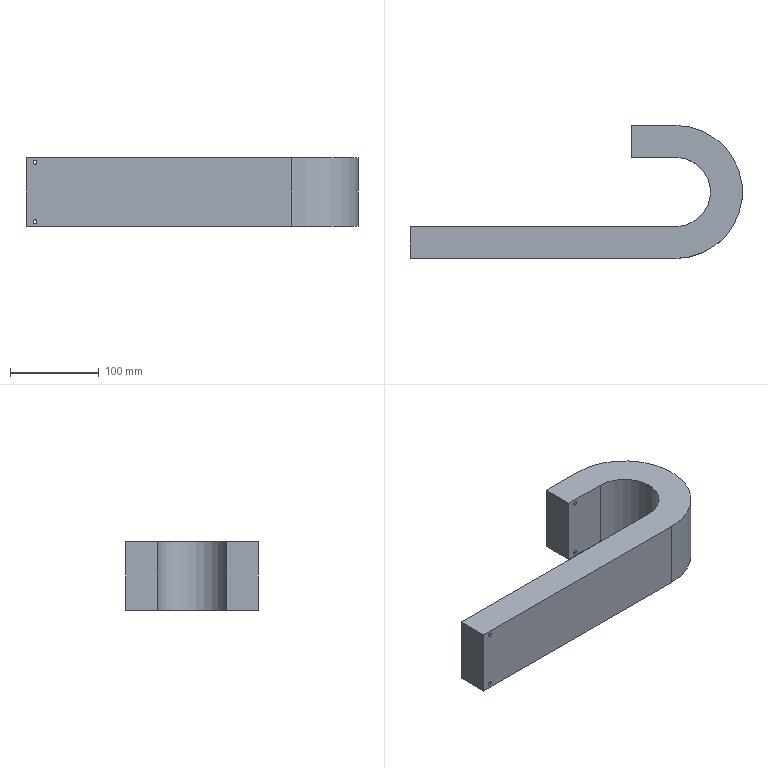Part | STEP file | 1 solid | 18 faces | box 375 x 150 x 77.5 mm | volume 1474112 mm3 | cylinder 10 | plane 8 | commonest cylinder face diameters 4.2 x8 78 x1 150 x1
STEP:
#1=CARTESIAN_POINT('',(0.,0.,0.));
#2=DIRECTION('',(0.,0.,1.));
#3=DIRECTION('',(1.,0.,0.));
#4=AXIS2_PLACEMENT_3D('',#1,#2,#3);
#5=CARTESIAN_POINT('',(-240.,36.,31.4));
#6=VERTEX_POINT('',#5);
#7=CARTESIAN_POINT('',(-240.,0.,31.4));
#8=VERTEX_POINT('',#7);
#9=CARTESIAN_POINT('',(-240.,0.,31.4));
#10=DIRECTION('',(0.,-1.,0.));
#11=VECTOR('',#10,1.);
#12=LINE('',#9,#11);
#13=CARTESIAN_POINT('',(-240.,0.,33.5));
#14=DIRECTION('',(0.,-1.,0.));
#15=DIRECTION('',(0.,0.,-1.));
#16=AXIS2_PLACEMENT_3D('',#13,#14,#15);
#17=CYLINDRICAL_SURFACE('',#16,2.1);
#18=CARTESIAN_POINT('',(6.283,0.));
#19=DIRECTION('',(0.,1.));
#20=VECTOR('',#19,1.);
#21=LINE('',#18,#20);
#22=(GEOMETRIC_REPRESENTATION_CONTEXT(2)PARAMETRIC_REPRESENTATION_CONTEXT()REPRESENTATION_CONTEXT('',''));
#23=DEFINITIONAL_REPRESENTATION('',(#21),#22);
#24=PCURVE('',#17,#23);
#25=CARTESIAN_POINT('',(-240.,0.,33.5));
#26=DIRECTION('',(0.,-1.,0.));
#27=DIRECTION('',(0.,0.,-1.));
#28=AXIS2_PLACEMENT_3D('',#25,#26,#27);
#29=CYLINDRICAL_SURFACE('',#28,2.1);
#30=CARTESIAN_POINT('',(0.,0.));
#31=DIRECTION('',(0.,1.));
#32=VECTOR('',#31,1.);
#33=LINE('',#30,#32);
#34=(GEOMETRIC_REPRESENTATION_CONTEXT(2)PARAMETRIC_REPRESENTATION_CONTEXT()REPRESENTATION_CONTEXT('',''));
#35=DEFINITIONAL_REPRESENTATION('',(#33),#34);
#36=PCURVE('',#29,#35);
#37=SURFACE_CURVE('',#12,(#24,#36),.PCURVE_S1.);
#38=EDGE_CURVE('',#6,#8,#37,.T.);
#39=ORIENTED_EDGE('',*,*,#38,.T.);
#40=CARTESIAN_POINT('',(-240.,0.,35.6));
#41=VERTEX_POINT('',#40);
#42=CARTESIAN_POINT('',(-240.,0.,33.5));
#43=DIRECTION('',(0.,-1.,0.));
#44=DIRECTION('',(0.,0.,-1.));
#45=AXIS2_PLACEMENT_3D('',#42,#43,#44);
#46=CIRCLE('',#45,2.1);
#47=CARTESIAN_POINT('',(0.,0.));
#48=DIRECTION('',(1.,0.));
#49=VECTOR('',#48,1.);
#50=LINE('',#47,#49);
#51=(GEOMETRIC_REPRESENTATION_CONTEXT(2)PARAMETRIC_REPRESENTATION_CONTEXT()REPRESENTATION_CONTEXT('',''));
#52=DEFINITIONAL_REPRESENTATION('',(#50),#51);
#53=PCURVE('',#17,#52);
#54=CARTESIAN_POINT('',(-250.,0.,38.75));
#55=DIRECTION('',(0.,1.,0.));
#56=DIRECTION('',(0.,0.,1.));
#57=AXIS2_PLACEMENT_3D('',#54,#55,#56);
#58=PLANE('',#57);
#59=CARTESIAN_POINT('',(-7.35,10.));
#60=CARTESIAN_POINT('',(-7.35,13.637));
#61=CARTESIAN_POINT('',(-4.2,11.819));
#62=CARTESIAN_POINT('',(-1.05,10.));
#63=CARTESIAN_POINT('',(-4.2,8.181));
#64=CARTESIAN_POINT('',(-7.35,6.363));
#65=CARTESIAN_POINT('',(-7.35,10.));
#66=(BOUNDED_CURVE()B_SPLINE_CURVE(2,(#59,#60,#61,#62,#63,#64,#65),.UNSPECIFIED.,.T.,.F.)B_SPLINE_CURVE_WITH_KNOTS((1,2,2,2,2,1),(-2.094,0.,2.094,4.189,6.283,8.378),.UNSPECIFIED.)CURVE()GEOMETRIC_REPRESENTATION_ITEM()RATIONAL_B_SPLINE_CURVE((1.,0.5,1.,0.5,1.,0.5,1.))REPRESENTATION_ITEM(''));
#67=(GEOMETRIC_REPRESENTATION_CONTEXT(2)PARAMETRIC_REPRESENTATION_CONTEXT()REPRESENTATION_CONTEXT('',''));
#68=DEFINITIONAL_REPRESENTATION('',(#66),#67);
#69=PCURVE('',#58,#68);
#70=SURFACE_CURVE('',#46,(#53,#69),.PCURVE_S1.);
#71=EDGE_CURVE('',#41,#8,#70,.T.);
#72=ORIENTED_EDGE('',*,*,#71,.F.);
#73=CARTESIAN_POINT('',(-240.,36.,35.6));
#74=VERTEX_POINT('',#73);
#75=CARTESIAN_POINT('',(-240.,0.,35.6));
#76=DIRECTION('',(0.,-1.,0.));
#77=VECTOR('',#76,1.);
#78=LINE('',#75,#77);
#79=CARTESIAN_POINT('',(3.142,0.));
#80=DIRECTION('',(0.,1.));
#81=VECTOR('',#80,1.);
#82=LINE('',#79,#81);
#83=(GEOMETRIC_REPRESENTATION_CONTEXT(2)PARAMETRIC_REPRESENTATION_CONTEXT()REPRESENTATION_CONTEXT('',''));
#84=DEFINITIONAL_REPRESENTATION('',(#82),#83);
#85=PCURVE('',#17,#84);
#86=CARTESIAN_POINT('',(3.142,0.));
#87=DIRECTION('',(0.,1.));
#88=VECTOR('',#87,1.);
#89=LINE('',#86,#88);
#90=(GEOMETRIC_REPRESENTATION_CONTEXT(2)PARAMETRIC_REPRESENTATION_CONTEXT()REPRESENTATION_CONTEXT('',''));
#91=DEFINITIONAL_REPRESENTATION('',(#89),#90);
#92=PCURVE('',#29,#91);
#93=SURFACE_CURVE('',#78,(#85,#92),.PCURVE_S1.);
#94=EDGE_CURVE('',#74,#41,#93,.T.);
#95=ORIENTED_EDGE('',*,*,#94,.F.);
#96=CARTESIAN_POINT('',(-240.,36.,33.5));
#97=DIRECTION('',(0.,-1.,0.));
#98=DIRECTION('',(0.,0.,-1.));
#99=AXIS2_PLACEMENT_3D('',#96,#97,#98);
#100=CIRCLE('',#99,2.1);
#101=CARTESIAN_POINT('',(0.,-36.));
#102=DIRECTION('',(1.,0.));
#103=VECTOR('',#102,1.);
#104=LINE('',#101,#103);
#105=(GEOMETRIC_REPRESENTATION_CONTEXT(2)PARAMETRIC_REPRESENTATION_CONTEXT()REPRESENTATION_CONTEXT('',''));
#106=DEFINITIONAL_REPRESENTATION('',(#104),#105);
#107=PCURVE('',#17,#106);
#108=CARTESIAN_POINT('',(-250.,36.,38.75));
#109=DIRECTION('',(0.,-1.,0.));
#110=DIRECTION('',(0.,0.,-1.));
#111=AXIS2_PLACEMENT_3D('',#108,#109,#110);
#112=PLANE('',#111);
#113=CARTESIAN_POINT('',(5.25,10.));
#114=DIRECTION('',(1.,0.));
#115=AXIS2_PLACEMENT_2D('',#113,#114);
#116=CIRCLE('',#115,2.1);
#117=(GEOMETRIC_REPRESENTATION_CONTEXT(2)PARAMETRIC_REPRESENTATION_CONTEXT()REPRESENTATION_CONTEXT('',''));
#118=DEFINITIONAL_REPRESENTATION('',(#116),#117);
#119=PCURVE('',#112,#118);
#120=SURFACE_CURVE('',#100,(#107,#119),.PCURVE_S1.);
#121=EDGE_CURVE('',#74,#6,#120,.T.);
#122=ORIENTED_EDGE('',*,*,#121,.T.);
#123=EDGE_LOOP('',(#39,#72,#95,#122));
#124=FACE_BOUND('',#123,.F.);
#125=ADVANCED_FACE('',(#124),#17,.F.);
#126=CARTESIAN_POINT('',(-240.,36.,-35.6));
#127=VERTEX_POINT('',#126);
#128=CARTESIAN_POINT('',(-240.,0.,-35.6));
#129=VERTEX_POINT('',#128);
#130=CARTESIAN_POINT('',(-240.,0.,-35.6));
#131=DIRECTION('',(0.,-1.,0.));
#132=VECTOR('',#131,1.);
#133=LINE('',#130,#132);
#134=CARTESIAN_POINT('',(-240.,0.,-33.5));
#135=DIRECTION('',(0.,-1.,0.));
#136=DIRECTION('',(0.,0.,-1.));
#137=AXIS2_PLACEMENT_3D('',#134,#135,#136);
#138=CYLINDRICAL_SURFACE('',#137,2.1);
#139=CARTESIAN_POINT('',(6.283,0.));
#140=DIRECTION('',(0.,1.));
#141=VECTOR('',#140,1.);
#142=LINE('',#139,#141);
#143=(GEOMETRIC_REPRESENTATION_CONTEXT(2)PARAMETRIC_REPRESENTATION_CONTEXT()REPRESENTATION_CONTEXT('',''));
#144=DEFINITIONAL_REPRESENTATION('',(#142),#143);
#145=PCURVE('',#138,#144);
#146=CARTESIAN_POINT('',(-240.,0.,-33.5));
#147=DIRECTION('',(0.,-1.,0.));
#148=DIRECTION('',(0.,0.,-1.));
#149=AXIS2_PLACEMENT_3D('',#146,#147,#148);
#150=CYLINDRICAL_SURFACE('',#149,2.1);
#151=CARTESIAN_POINT('',(0.,0.));
#152=DIRECTION('',(0.,1.));
#153=VECTOR('',#152,1.);
#154=LINE('',#151,#153);
#155=(GEOMETRIC_REPRESENTATION_CONTEXT(2)PARAMETRIC_REPRESENTATION_CONTEXT()REPRESENTATION_CONTEXT('',''));
#156=DEFINITIONAL_REPRESENTATION('',(#154),#155);
#157=PCURVE('',#150,#156);
#158=SURFACE_CURVE('',#133,(#145,#157),.PCURVE_S1.);
#159=EDGE_CURVE('',#127,#129,#158,.T.);
#160=ORIENTED_EDGE('',*,*,#159,.T.);
#161=CARTESIAN_POINT('',(-240.,0.,-31.4));
#162=VERTEX_POINT('',#161);
#163=CARTESIAN_POINT('',(-240.,0.,-33.5));
#164=DIRECTION('',(0.,-1.,0.));
#165=DIRECTION('',(0.,0.,-1.));
#166=AXIS2_PLACEMENT_3D('',#163,#164,#165);
#167=CIRCLE('',#166,2.1);
#168=CARTESIAN_POINT('',(0.,0.));
#169=DIRECTION('',(1.,0.));
#170=VECTOR('',#169,1.);
#171=LINE('',#168,#170);
#172=(GEOMETRIC_REPRESENTATION_CONTEXT(2)PARAMETRIC_REPRESENTATION_CONTEXT()REPRESENTATION_CONTEXT('',''));
#173=DEFINITIONAL_REPRESENTATION('',(#171),#172);
#174=PCURVE('',#138,#173);
#175=CARTESIAN_POINT('',(-74.35,10.));
#176=CARTESIAN_POINT('',(-74.35,13.637));
#177=CARTESIAN_POINT('',(-71.2,11.819));
#178=CARTESIAN_POINT('',(-68.05,10.));
#179=CARTESIAN_POINT('',(-71.2,8.181));
#180=CARTESIAN_POINT('',(-74.35,6.363));
#181=CARTESIAN_POINT('',(-74.35,10.));
#182=(BOUNDED_CURVE()B_SPLINE_CURVE(2,(#175,#176,#177,#178,#179,#180,#181),.UNSPECIFIED.,.T.,.F.)B_SPLINE_CURVE_WITH_KNOTS((1,2,2,2,2,1),(-2.094,0.,2.094,4.189,6.283,8.378),.UNSPECIFIED.)CURVE()GEOMETRIC_REPRESENTATION_ITEM()RATIONAL_B_SPLINE_CURVE((1.,0.5,1.,0.5,1.,0.5,1.))REPRESENTATION_ITEM(''));
#183=(GEOMETRIC_REPRESENTATION_CONTEXT(2)PARAMETRIC_REPRESENTATION_CONTEXT()REPRESENTATION_CONTEXT('',''));
#184=DEFINITIONAL_REPRESENTATION('',(#182),#183);
#185=PCURVE('',#58,#184);
#186=SURFACE_CURVE('',#167,(#174,#185),.PCURVE_S1.);
#187=EDGE_CURVE('',#162,#129,#186,.T.);
#188=ORIENTED_EDGE('',*,*,#187,.F.);
#189=CARTESIAN_POINT('',(-240.,36.,-31.4));
#190=VERTEX_POINT('',#189);
#191=CARTESIAN_POINT('',(-240.,0.,-31.4));
#192=DIRECTION('',(0.,-1.,0.));
#193=VECTOR('',#192,1.);
#194=LINE('',#191,#193);
#195=CARTESIAN_POINT('',(3.142,0.));
#196=DIRECTION('',(0.,1.));
#197=VECTOR('',#196,1.);
#198=LINE('',#195,#197);
#199=(GEOMETRIC_REPRESENTATION_CONTEXT(2)PARAMETRIC_REPRESENTATION_CONTEXT()REPRESENTATION_CONTEXT('',''));
#200=DEFINITIONAL_REPRESENTATION('',(#198),#199);
#201=PCURVE('',#138,#200);
#202=CARTESIAN_POINT('',(3.142,0.));
#203=DIRECTION('',(0.,1.));
#204=VECTOR('',#203,1.);
#205=LINE('',#202,#204);
#206=(GEOMETRIC_REPRESENTATION_CONTEXT(2)PARAMETRIC_REPRESENTATION_CONTEXT()REPRESENTATION_CONTEXT('',''));
#207=DEFINITIONAL_REPRESENTATION('',(#205),#206);
#208=PCURVE('',#150,#207);
#209=SURFACE_CURVE('',#194,(#201,#208),.PCURVE_S1.);
#210=EDGE_CURVE('',#190,#162,#209,.T.);
#211=ORIENTED_EDGE('',*,*,#210,.F.);
#212=CARTESIAN_POINT('',(-240.,36.,-33.5));
#213=DIRECTION('',(0.,-1.,0.));
#214=DIRECTION('',(0.,0.,-1.));
#215=AXIS2_PLACEMENT_3D('',#212,#213,#214);
#216=CIRCLE('',#215,2.1);
#217=CARTESIAN_POINT('',(0.,-36.));
#218=DIRECTION('',(1.,0.));
#219=VECTOR('',#218,1.);
#220=LINE('',#217,#219);
#221=(GEOMETRIC_REPRESENTATION_CONTEXT(2)PARAMETRIC_REPRESENTATION_CONTEXT()REPRESENTATION_CONTEXT('',''));
#222=DEFINITIONAL_REPRESENTATION('',(#220),#221);
#223=PCURVE('',#138,#222);
#224=CARTESIAN_POINT('',(72.25,10.));
#225=DIRECTION('',(1.,0.));
#226=AXIS2_PLACEMENT_2D('',#224,#225);
#227=CIRCLE('',#226,2.1);
#228=(GEOMETRIC_REPRESENTATION_CONTEXT(2)PARAMETRIC_REPRESENTATION_CONTEXT()REPRESENTATION_CONTEXT('',''));
#229=DEFINITIONAL_REPRESENTATION('',(#227),#228);
#230=PCURVE('',#112,#229);
#231=SURFACE_CURVE('',#216,(#223,#230),.PCURVE_S1.);
#232=EDGE_CURVE('',#190,#127,#231,.T.);
#233=ORIENTED_EDGE('',*,*,#232,.T.);
#234=EDGE_LOOP('',(#160,#188,#211,#233));
#235=FACE_BOUND('',#234,.F.);
#236=ADVANCED_FACE('',(#235),#138,.F.);
#237=CARTESIAN_POINT('',(10.,150.,31.4));
#238=VERTEX_POINT('',#237);
#239=CARTESIAN_POINT('',(10.,114.,31.4));
#240=VERTEX_POINT('',#239);
#241=CARTESIAN_POINT('',(10.,114.,31.4));
#242=DIRECTION('',(0.,-1.,0.));
#243=VECTOR('',#242,1.);
#244=LINE('',#241,#243);
#245=CARTESIAN_POINT('',(10.,114.,33.5));
#246=DIRECTION('',(0.,-1.,0.));
#247=DIRECTION('',(0.,0.,-1.));
#248=AXIS2_PLACEMENT_3D('',#245,#246,#247);
#249=CYLINDRICAL_SURFACE('',#248,2.1);
#250=CARTESIAN_POINT('',(6.283,0.));
#251=DIRECTION('',(0.,1.));
#252=VECTOR('',#251,1.);
#253=LINE('',#250,#252);
#254=(GEOMETRIC_REPRESENTATION_CONTEXT(2)PARAMETRIC_REPRESENTATION_CONTEXT()REPRESENTATION_CONTEXT('',''));
#255=DEFINITIONAL_REPRESENTATION('',(#253),#254);
#256=PCURVE('',#249,#255);
#257=CARTESIAN_POINT('',(10.,114.,33.5));
#258=DIRECTION('',(0.,-1.,0.));
#259=DIRECTION('',(0.,0.,-1.));
#260=AXIS2_PLACEMENT_3D('',#257,#258,#259);
#261=CYLINDRICAL_SURFACE('',#260,2.1);
#262=CARTESIAN_POINT('',(0.,0.));
#263=DIRECTION('',(0.,1.));
#264=VECTOR('',#263,1.);
#265=LINE('',#262,#264);
#266=(GEOMETRIC_REPRESENTATION_CONTEXT(2)PARAMETRIC_REPRESENTATION_CONTEXT()REPRESENTATION_CONTEXT('',''));
#267=DEFINITIONAL_REPRESENTATION('',(#265),#266);
#268=PCURVE('',#261,#267);
#269=SURFACE_CURVE('',#244,(#256,#268),.PCURVE_S1.);
#270=EDGE_CURVE('',#238,#240,#269,.T.);
#271=ORIENTED_EDGE('',*,*,#270,.T.);
#272=CARTESIAN_POINT('',(10.,114.,35.6));
#273=VERTEX_POINT('',#272);
#274=CARTESIAN_POINT('',(10.,114.,33.5));
#275=DIRECTION('',(0.,-1.,0.));
#276=DIRECTION('',(0.,0.,-1.));
#277=AXIS2_PLACEMENT_3D('',#274,#275,#276);
#278=CIRCLE('',#277,2.1);
#279=CARTESIAN_POINT('',(0.,0.));
#280=DIRECTION('',(1.,0.));
#281=VECTOR('',#280,1.);
#282=LINE('',#279,#281);
#283=(GEOMETRIC_REPRESENTATION_CONTEXT(2)PARAMETRIC_REPRESENTATION_CONTEXT()REPRESENTATION_CONTEXT('',''));
#284=DEFINITIONAL_REPRESENTATION('',(#282),#283);
#285=PCURVE('',#249,#284);
#286=CARTESIAN_POINT('',(0.,114.,38.75));
#287=DIRECTION('',(0.,1.,0.));
#288=DIRECTION('',(-1.,0.,0.));
#289=AXIS2_PLACEMENT_3D('',#286,#287,#288);
#290=PLANE('',#289);
#291=CARTESIAN_POINT('',(-10.,-7.35));
#292=CARTESIAN_POINT('',(-13.637,-7.35));
#293=CARTESIAN_POINT('',(-11.819,-4.2));
#294=CARTESIAN_POINT('',(-10.,-1.05));
#295=CARTESIAN_POINT('',(-8.181,-4.2));
#296=CARTESIAN_POINT('',(-6.363,-7.35));
#297=CARTESIAN_POINT('',(-10.,-7.35));
#298=(BOUNDED_CURVE()B_SPLINE_CURVE(2,(#291,#292,#293,#294,#295,#296,#297),.UNSPECIFIED.,.T.,.F.)B_SPLINE_CURVE_WITH_KNOTS((1,2,2,2,2,1),(-2.094,0.,2.094,4.189,6.283,8.378),.UNSPECIFIED.)CURVE()GEOMETRIC_REPRESENTATION_ITEM()RATIONAL_B_SPLINE_CURVE((1.,0.5,1.,0.5,1.,0.5,1.))REPRESENTATION_ITEM(''));
#299=(GEOMETRIC_REPRESENTATION_CONTEXT(2)PARAMETRIC_REPRESENTATION_CONTEXT()REPRESENTATION_CONTEXT('',''));
#300=DEFINITIONAL_REPRESENTATION('',(#298),#299);
#301=PCURVE('',#290,#300);
#302=SURFACE_CURVE('',#278,(#285,#301),.PCURVE_S1.);
#303=EDGE_CURVE('',#273,#240,#302,.T.);
#304=ORIENTED_EDGE('',*,*,#303,.F.);
#305=CARTESIAN_POINT('',(10.,150.,35.6));
#306=VERTEX_POINT('',#305);
#307=CARTESIAN_POINT('',(10.,114.,35.6));
#308=DIRECTION('',(0.,-1.,0.));
#309=VECTOR('',#308,1.);
#310=LINE('',#307,#309);
#311=CARTESIAN_POINT('',(3.142,0.));
#312=DIRECTION('',(0.,1.));
#313=VECTOR('',#312,1.);
#314=LINE('',#311,#313);
#315=(GEOMETRIC_REPRESENTATION_CONTEXT(2)PARAMETRIC_REPRESENTATION_CONTEXT()REPRESENTATION_CONTEXT('',''));
#316=DEFINITIONAL_REPRESENTATION('',(#314),#315);
#317=PCURVE('',#249,#316);
#318=CARTESIAN_POINT('',(3.142,0.));
#319=DIRECTION('',(0.,1.));
#320=VECTOR('',#319,1.);
#321=LINE('',#318,#320);
#322=(GEOMETRIC_REPRESENTATION_CONTEXT(2)PARAMETRIC_REPRESENTATION_CONTEXT()REPRESENTATION_CONTEXT('',''));
#323=DEFINITIONAL_REPRESENTATION('',(#321),#322);
#324=PCURVE('',#261,#323);
#325=SURFACE_CURVE('',#310,(#317,#324),.PCURVE_S1.);
#326=EDGE_CURVE('',#306,#273,#325,.T.);
#327=ORIENTED_EDGE('',*,*,#326,.F.);
#328=CARTESIAN_POINT('',(10.,150.,33.5));
#329=DIRECTION('',(0.,-1.,0.));
#330=DIRECTION('',(0.,0.,-1.));
#331=AXIS2_PLACEMENT_3D('',#328,#329,#330);
#332=CIRCLE('',#331,2.1);
#333=CARTESIAN_POINT('',(0.,-36.));
#334=DIRECTION('',(1.,0.));
#335=VECTOR('',#334,1.);
#336=LINE('',#333,#335);
#337=(GEOMETRIC_REPRESENTATION_CONTEXT(2)PARAMETRIC_REPRESENTATION_CONTEXT()REPRESENTATION_CONTEXT('',''));
#338=DEFINITIONAL_REPRESENTATION('',(#336),#337);
#339=PCURVE('',#249,#338);
#340=CARTESIAN_POINT('',(0.,150.,38.75));
#341=DIRECTION('',(0.,-1.,0.));
#342=DIRECTION('',(0.,0.,-1.));
#343=AXIS2_PLACEMENT_3D('',#340,#341,#342);
#344=PLANE('',#343);
#345=CARTESIAN_POINT('',(5.25,10.));
#346=DIRECTION('',(1.,0.));
#347=AXIS2_PLACEMENT_2D('',#345,#346);
#348=CIRCLE('',#347,2.1);
#349=(GEOMETRIC_REPRESENTATION_CONTEXT(2)PARAMETRIC_REPRESENTATION_CONTEXT()REPRESENTATION_CONTEXT('',''));
#350=DEFINITIONAL_REPRESENTATION('',(#348),#349);
#351=PCURVE('',#344,#350);
#352=SURFACE_CURVE('',#332,(#339,#351),.PCURVE_S1.);
#353=EDGE_CURVE('',#306,#238,#352,.T.);
#354=ORIENTED_EDGE('',*,*,#353,.T.);
#355=EDGE_LOOP('',(#271,#304,#327,#354));
#356=FACE_BOUND('',#355,.F.);
#357=ADVANCED_FACE('',(#356),#249,.F.);
#358=CARTESIAN_POINT('',(10.,150.,-35.6));
#359=VERTEX_POINT('',#358);
#360=CARTESIAN_POINT('',(10.,114.,-35.6));
#361=VERTEX_POINT('',#360);
#362=CARTESIAN_POINT('',(10.,114.,-35.6));
#363=DIRECTION('',(0.,-1.,0.));
#364=VECTOR('',#363,1.);
#365=LINE('',#362,#364);
#366=CARTESIAN_POINT('',(10.,114.,-33.5));
#367=DIRECTION('',(0.,-1.,0.));
#368=DIRECTION('',(0.,0.,-1.));
#369=AXIS2_PLACEMENT_3D('',#366,#367,#368);
#370=CYLINDRICAL_SURFACE('',#369,2.1);
#371=CARTESIAN_POINT('',(6.283,0.));
#372=DIRECTION('',(0.,1.));
#373=VECTOR('',#372,1.);
#374=LINE('',#371,#373);
#375=(GEOMETRIC_REPRESENTATION_CONTEXT(2)PARAMETRIC_REPRESENTATION_CONTEXT()REPRESENTATION_CONTEXT('',''));
#376=DEFINITIONAL_REPRESENTATION('',(#374),#375);
#377=PCURVE('',#370,#376);
#378=CARTESIAN_POINT('',(10.,114.,-33.5));
#379=DIRECTION('',(0.,-1.,0.));
#380=DIRECTION('',(0.,0.,-1.));
#381=AXIS2_PLACEMENT_3D('',#378,#379,#380);
#382=CYLINDRICAL_SURFACE('',#381,2.1);
#383=CARTESIAN_POINT('',(0.,0.));
#384=DIRECTION('',(0.,1.));
#385=VECTOR('',#384,1.);
#386=LINE('',#383,#385);
#387=(GEOMETRIC_REPRESENTATION_CONTEXT(2)PARAMETRIC_REPRESENTATION_CONTEXT()REPRESENTATION_CONTEXT('',''));
#388=DEFINITIONAL_REPRESENTATION('',(#386),#387);
#389=PCURVE('',#382,#388);
#390=SURFACE_CURVE('',#365,(#377,#389),.PCURVE_S1.);
#391=EDGE_CURVE('',#359,#361,#390,.T.);
#392=ORIENTED_EDGE('',*,*,#391,.T.);
#393=CARTESIAN_POINT('',(10.,114.,-31.4));
#394=VERTEX_POINT('',#393);
#395=CARTESIAN_POINT('',(10.,114.,-33.5));
#396=DIRECTION('',(0.,-1.,0.));
#397=DIRECTION('',(0.,0.,-1.));
#398=AXIS2_PLACEMENT_3D('',#395,#396,#397);
#399=CIRCLE('',#398,2.1);
#400=CARTESIAN_POINT('',(0.,0.));
#401=DIRECTION('',(1.,0.));
#402=VECTOR('',#401,1.);
#403=LINE('',#400,#402);
#404=(GEOMETRIC_REPRESENTATION_CONTEXT(2)PARAMETRIC_REPRESENTATION_CONTEXT()REPRESENTATION_CONTEXT('',''));
#405=DEFINITIONAL_REPRESENTATION('',(#403),#404);
#406=PCURVE('',#370,#405);
#407=CARTESIAN_POINT('',(-10.,-74.35));
#408=CARTESIAN_POINT('',(-13.637,-74.35));
#409=CARTESIAN_POINT('',(-11.819,-71.2));
#410=CARTESIAN_POINT('',(-10.,-68.05));
#411=CARTESIAN_POINT('',(-8.181,-71.2));
#412=CARTESIAN_POINT('',(-6.363,-74.35));
#413=CARTESIAN_POINT('',(-10.,-74.35));
#414=(BOUNDED_CURVE()B_SPLINE_CURVE(2,(#407,#408,#409,#410,#411,#412,#413),.UNSPECIFIED.,.T.,.F.)B_SPLINE_CURVE_WITH_KNOTS((1,2,2,2,2,1),(-2.094,0.,2.094,4.189,6.283,8.378),.UNSPECIFIED.)CURVE()GEOMETRIC_REPRESENTATION_ITEM()RATIONAL_B_SPLINE_CURVE((1.,0.5,1.,0.5,1.,0.5,1.))REPRESENTATION_ITEM(''));
#415=(GEOMETRIC_REPRESENTATION_CONTEXT(2)PARAMETRIC_REPRESENTATION_CONTEXT()REPRESENTATION_CONTEXT('',''));
#416=DEFINITIONAL_REPRESENTATION('',(#414),#415);
#417=PCURVE('',#290,#416);
#418=SURFACE_CURVE('',#399,(#406,#417),.PCURVE_S1.);
#419=EDGE_CURVE('',#394,#361,#418,.T.);
#420=ORIENTED_EDGE('',*,*,#419,.F.);
#421=CARTESIAN_POINT('',(10.,150.,-31.4));
#422=VERTEX_POINT('',#421);
#423=CARTESIAN_POINT('',(10.,114.,-31.4));
#424=DIRECTION('',(0.,-1.,0.));
#425=VECTOR('',#424,1.);
#426=LINE('',#423,#425);
#427=CARTESIAN_POINT('',(3.142,0.));
#428=DIRECTION('',(0.,1.));
#429=VECTOR('',#428,1.);
#430=LINE('',#427,#429);
#431=(GEOMETRIC_REPRESENTATION_CONTEXT(2)PARAMETRIC_REPRESENTATION_CONTEXT()REPRESENTATION_CONTEXT('',''));
#432=DEFINITIONAL_REPRESENTATION('',(#430),#431);
#433=PCURVE('',#370,#432);
#434=CARTESIAN_POINT('',(3.142,0.));
#435=DIRECTION('',(0.,1.));
#436=VECTOR('',#435,1.);
#437=LINE('',#434,#436);
#438=(GEOMETRIC_REPRESENTATION_CONTEXT(2)PARAMETRIC_REPRESENTATION_CONTEXT()REPRESENTATION_CONTEXT('',''));
#439=DEFINITIONAL_REPRESENTATION('',(#437),#438);
#440=PCURVE('',#382,#439);
#441=SURFACE_CURVE('',#426,(#433,#440),.PCURVE_S1.);
#442=EDGE_CURVE('',#422,#394,#441,.T.);
#443=ORIENTED_EDGE('',*,*,#442,.F.);
#444=CARTESIAN_POINT('',(10.,150.,-33.5));
#445=DIRECTION('',(0.,-1.,0.));
#446=DIRECTION('',(0.,0.,-1.));
#447=AXIS2_PLACEMENT_3D('',#444,#445,#446);
#448=CIRCLE('',#447,2.1);
#449=CARTESIAN_POINT('',(0.,-36.));
#450=DIRECTION('',(1.,0.));
#451=VECTOR('',#450,1.);
#452=LINE('',#449,#451);
#453=(GEOMETRIC_REPRESENTATION_CONTEXT(2)PARAMETRIC_REPRESENTATION_CONTEXT()REPRESENTATION_CONTEXT('',''));
#454=DEFINITIONAL_REPRESENTATION('',(#452),#453);
#455=PCURVE('',#370,#454);
#456=CARTESIAN_POINT('',(72.25,10.));
#457=DIRECTION('',(1.,0.));
#458=AXIS2_PLACEMENT_2D('',#456,#457);
#459=CIRCLE('',#458,2.1);
#460=(GEOMETRIC_REPRESENTATION_CONTEXT(2)PARAMETRIC_REPRESENTATION_CONTEXT()REPRESENTATION_CONTEXT('',''));
#461=DEFINITIONAL_REPRESENTATION('',(#459),#460);
#462=PCURVE('',#344,#461);
#463=SURFACE_CURVE('',#448,(#455,#462),.PCURVE_S1.);
#464=EDGE_CURVE('',#422,#359,#463,.T.);
#465=ORIENTED_EDGE('',*,*,#464,.T.);
#466=EDGE_LOOP('',(#392,#420,#443,#465));
#467=FACE_BOUND('',#466,.F.);
#468=ADVANCED_FACE('',(#467),#370,.F.);
#469=CARTESIAN_POINT('',(0.,150.,-38.75));
#470=VERTEX_POINT('',#469);
#471=CARTESIAN_POINT('',(0.,114.,-38.75));
#472=VERTEX_POINT('',#471);
#473=CARTESIAN_POINT('',(0.,114.,-38.75));
#474=DIRECTION('',(0.,-1.,0.));
#475=VECTOR('',#474,1.);
#476=LINE('',#473,#475);
#477=CARTESIAN_POINT('',(0.,114.,38.75));
#478=DIRECTION('',(1.,0.,0.));
#479=DIRECTION('',(0.,0.,-1.));
#480=AXIS2_PLACEMENT_3D('',#477,#478,#479);
#481=PLANE('',#480);
#482=CARTESIAN_POINT('',(77.5,0.));
#483=DIRECTION('',(0.,-1.));
#484=VECTOR('',#483,1.);
#485=LINE('',#482,#484);
#486=(GEOMETRIC_REPRESENTATION_CONTEXT(2)PARAMETRIC_REPRESENTATION_CONTEXT()REPRESENTATION_CONTEXT('',''));
#487=DEFINITIONAL_REPRESENTATION('',(#485),#486);
#488=PCURVE('',#481,#487);
#489=CARTESIAN_POINT('',(50.,75.,-38.75));
#490=DIRECTION('',(0.,0.,-1.));
#491=DIRECTION('',(-1.,0.,0.));
#492=AXIS2_PLACEMENT_3D('',#489,#490,#491);
#493=PLANE('',#492);
#494=CARTESIAN_POINT('',(50.,39.));
#495=DIRECTION('',(0.,-1.));
#496=VECTOR('',#495,1.);
#497=LINE('',#494,#496);
#498=(GEOMETRIC_REPRESENTATION_CONTEXT(2)PARAMETRIC_REPRESENTATION_CONTEXT()REPRESENTATION_CONTEXT('',''));
#499=DEFINITIONAL_REPRESENTATION('',(#497),#498);
#500=PCURVE('',#493,#499);
#501=SURFACE_CURVE('',#476,(#488,#500),.PCURVE_S1.);
#502=EDGE_CURVE('',#470,#472,#501,.T.);
#503=ORIENTED_EDGE('',*,*,#502,.T.);
#504=CARTESIAN_POINT('',(0.,114.,38.75));
#505=VERTEX_POINT('',#504);
#506=CARTESIAN_POINT('',(0.,114.,38.75));
#507=DIRECTION('',(0.,0.,-1.));
#508=VECTOR('',#507,1.);
#509=LINE('',#506,#508);
#510=CARTESIAN_POINT('',(0.,0.));
#511=DIRECTION('',(1.,0.));
#512=VECTOR('',#511,1.);
#513=LINE('',#510,#512);
#514=(GEOMETRIC_REPRESENTATION_CONTEXT(2)PARAMETRIC_REPRESENTATION_CONTEXT()REPRESENTATION_CONTEXT('',''));
#515=DEFINITIONAL_REPRESENTATION('',(#513),#514);
#516=PCURVE('',#481,#515);
#517=CARTESIAN_POINT('',(0.,0.));
#518=DIRECTION('',(0.,-1.));
#519=VECTOR('',#518,1.);
#520=LINE('',#517,#519);
#521=(GEOMETRIC_REPRESENTATION_CONTEXT(2)PARAMETRIC_REPRESENTATION_CONTEXT()REPRESENTATION_CONTEXT('',''));
#522=DEFINITIONAL_REPRESENTATION('',(#520),#521);
#523=PCURVE('',#290,#522);
#524=SURFACE_CURVE('',#509,(#516,#523),.PCURVE_S1.);
#525=EDGE_CURVE('',#505,#472,#524,.T.);
#526=ORIENTED_EDGE('',*,*,#525,.F.);
#527=CARTESIAN_POINT('',(0.,150.,38.75));
#528=VERTEX_POINT('',#527);
#529=CARTESIAN_POINT('',(0.,114.,38.75));
#530=DIRECTION('',(0.,-1.,0.));
#531=VECTOR('',#530,1.);
#532=LINE('',#529,#531);
#533=CARTESIAN_POINT('',(0.,0.));
#534=DIRECTION('',(0.,-1.));
#535=VECTOR('',#534,1.);
#536=LINE('',#533,#535);
#537=(GEOMETRIC_REPRESENTATION_CONTEXT(2)PARAMETRIC_REPRESENTATION_CONTEXT()REPRESENTATION_CONTEXT('',''));
#538=DEFINITIONAL_REPRESENTATION('',(#536),#537);
#539=PCURVE('',#481,#538);
#540=CARTESIAN_POINT('',(50.,75.,38.75));
#541=DIRECTION('',(0.,0.,-1.));
#542=DIRECTION('',(-1.,0.,0.));
#543=AXIS2_PLACEMENT_3D('',#540,#541,#542);
#544=PLANE('',#543);
#545=CARTESIAN_POINT('',(50.,39.));
#546=DIRECTION('',(0.,-1.));
#547=VECTOR('',#546,1.);
#548=LINE('',#545,#547);
#549=(GEOMETRIC_REPRESENTATION_CONTEXT(2)PARAMETRIC_REPRESENTATION_CONTEXT()REPRESENTATION_CONTEXT('',''));
#550=DEFINITIONAL_REPRESENTATION('',(#548),#549);
#551=PCURVE('',#544,#550);
#552=SURFACE_CURVE('',#532,(#539,#551),.PCURVE_S1.);
#553=EDGE_CURVE('',#528,#505,#552,.T.);
#554=ORIENTED_EDGE('',*,*,#553,.F.);
#555=CARTESIAN_POINT('',(0.,150.,38.75));
#556=DIRECTION('',(0.,0.,-1.));
#557=VECTOR('',#556,1.);
#558=LINE('',#555,#557);
#559=CARTESIAN_POINT('',(0.,36.));
#560=DIRECTION('',(1.,0.));
#561=VECTOR('',#560,1.);
#562=LINE('',#559,#561);
#563=(GEOMETRIC_REPRESENTATION_CONTEXT(2)PARAMETRIC_REPRESENTATION_CONTEXT()REPRESENTATION_CONTEXT('',''));
#564=DEFINITIONAL_REPRESENTATION('',(#562),#563);
#565=PCURVE('',#481,#564);
#566=CARTESIAN_POINT('',(0.,0.));
#567=DIRECTION('',(1.,0.));
#568=VECTOR('',#567,1.);
#569=LINE('',#566,#568);
#570=(GEOMETRIC_REPRESENTATION_CONTEXT(2)PARAMETRIC_REPRESENTATION_CONTEXT()REPRESENTATION_CONTEXT('',''));
#571=DEFINITIONAL_REPRESENTATION('',(#569),#570);
#572=PCURVE('',#344,#571);
#573=SURFACE_CURVE('',#558,(#565,#572),.PCURVE_S1.);
#574=EDGE_CURVE('',#528,#470,#573,.T.);
#575=ORIENTED_EDGE('',*,*,#574,.T.);
#576=EDGE_LOOP('',(#503,#526,#554,#575));
#577=FACE_BOUND('',#576,.T.);
#578=ADVANCED_FACE('',(#577),#481,.F.);
#579=CARTESIAN_POINT('',(10.,114.,33.5));
#580=DIRECTION('',(0.,-1.,0.));
#581=DIRECTION('',(0.,0.,-1.));
#582=AXIS2_PLACEMENT_3D('',#579,#580,#581);
#583=CIRCLE('',#582,2.1);
#584=CARTESIAN_POINT('',(-10.,-7.35));
#585=CARTESIAN_POINT('',(-13.637,-7.35));
#586=CARTESIAN_POINT('',(-11.819,-4.2));
#587=CARTESIAN_POINT('',(-10.,-1.05));
#588=CARTESIAN_POINT('',(-8.181,-4.2));
#589=CARTESIAN_POINT('',(-6.363,-7.35));
#590=CARTESIAN_POINT('',(-10.,-7.35));
#591=(BOUNDED_CURVE()B_SPLINE_CURVE(2,(#584,#585,#586,#587,#588,#589,#590),.UNSPECIFIED.,.T.,.F.)B_SPLINE_CURVE_WITH_KNOTS((1,2,2,2,2,1),(-2.094,0.,2.094,4.189,6.283,8.378),.UNSPECIFIED.)CURVE()GEOMETRIC_REPRESENTATION_ITEM()RATIONAL_B_SPLINE_CURVE((1.,0.5,1.,0.5,1.,0.5,1.))REPRESENTATION_ITEM(''));
#592=(GEOMETRIC_REPRESENTATION_CONTEXT(2)PARAMETRIC_REPRESENTATION_CONTEXT()REPRESENTATION_CONTEXT('',''));
#593=DEFINITIONAL_REPRESENTATION('',(#591),#592);
#594=PCURVE('',#290,#593);
#595=CARTESIAN_POINT('',(0.,0.));
#596=DIRECTION('',(1.,0.));
#597=VECTOR('',#596,1.);
#598=LINE('',#595,#597);
#599=(GEOMETRIC_REPRESENTATION_CONTEXT(2)PARAMETRIC_REPRESENTATION_CONTEXT()REPRESENTATION_CONTEXT('',''));
#600=DEFINITIONAL_REPRESENTATION('',(#598),#599);
#601=PCURVE('',#261,#600);
#602=SURFACE_CURVE('',#583,(#594,#601),.PCURVE_S1.);
#603=EDGE_CURVE('',#240,#273,#602,.T.);
#604=ORIENTED_EDGE('',*,*,#603,.F.);
#605=ORIENTED_EDGE('',*,*,#303,.F.);
#606=EDGE_LOOP('',(#604,#605));
#607=FACE_BOUND('',#606,.T.);
#608=CARTESIAN_POINT('',(10.,114.,-33.5));
#609=DIRECTION('',(0.,-1.,0.));
#610=DIRECTION('',(0.,0.,-1.));
#611=AXIS2_PLACEMENT_3D('',#608,#609,#610);
#612=CIRCLE('',#611,2.1);
#613=CARTESIAN_POINT('',(-10.,-74.35));
#614=CARTESIAN_POINT('',(-13.637,-74.35));
#615=CARTESIAN_POINT('',(-11.819,-71.2));
#616=CARTESIAN_POINT('',(-10.,-68.05));
#617=CARTESIAN_POINT('',(-8.181,-71.2));
#618=CARTESIAN_POINT('',(-6.363,-74.35));
#619=CARTESIAN_POINT('',(-10.,-74.35));
#620=(BOUNDED_CURVE()B_SPLINE_CURVE(2,(#613,#614,#615,#616,#617,#618,#619),.UNSPECIFIED.,.T.,.F.)B_SPLINE_CURVE_WITH_KNOTS((1,2,2,2,2,1),(-2.094,0.,2.094,4.189,6.283,8.378),.UNSPECIFIED.)CURVE()GEOMETRIC_REPRESENTATION_ITEM()RATIONAL_B_SPLINE_CURVE((1.,0.5,1.,0.5,1.,0.5,1.))REPRESENTATION_ITEM(''));
#621=(GEOMETRIC_REPRESENTATION_CONTEXT(2)PARAMETRIC_REPRESENTATION_CONTEXT()REPRESENTATION_CONTEXT('',''));
#622=DEFINITIONAL_REPRESENTATION('',(#620),#621);
#623=PCURVE('',#290,#622);
#624=CARTESIAN_POINT('',(0.,0.));
#625=DIRECTION('',(1.,0.));
#626=VECTOR('',#625,1.);
#627=LINE('',#624,#626);
#628=(GEOMETRIC_REPRESENTATION_CONTEXT(2)PARAMETRIC_REPRESENTATION_CONTEXT()REPRESENTATION_CONTEXT('',''));
#629=DEFINITIONAL_REPRESENTATION('',(#627),#628);
#630=PCURVE('',#382,#629);
#631=SURFACE_CURVE('',#612,(#623,#630),.PCURVE_S1.);
#632=EDGE_CURVE('',#361,#394,#631,.T.);
#633=ORIENTED_EDGE('',*,*,#632,.F.);
#634=ORIENTED_EDGE('',*,*,#419,.F.);
#635=EDGE_LOOP('',(#633,#634));
#636=FACE_BOUND('',#635,.T.);
#637=CARTESIAN_POINT('',(50.,114.,-38.75));
#638=VERTEX_POINT('',#637);
#639=CARTESIAN_POINT('',(0.,114.,-38.75));
#640=DIRECTION('',(1.,0.,0.));
#641=VECTOR('',#640,1.);
#642=LINE('',#639,#641);
#643=CARTESIAN_POINT('',(0.,-77.5));
#644=DIRECTION('',(-1.,0.));
#645=VECTOR('',#644,1.);
#646=LINE('',#643,#645);
#647=(GEOMETRIC_REPRESENTATION_CONTEXT(2)PARAMETRIC_REPRESENTATION_CONTEXT()REPRESENTATION_CONTEXT('',''));
#648=DEFINITIONAL_REPRESENTATION('',(#646),#647);
#649=PCURVE('',#290,#648);
#650=CARTESIAN_POINT('',(50.,39.));
#651=DIRECTION('',(-1.,0.));
#652=VECTOR('',#651,1.);
#653=LINE('',#650,#652);
#654=(GEOMETRIC_REPRESENTATION_CONTEXT(2)PARAMETRIC_REPRESENTATION_CONTEXT()REPRESENTATION_CONTEXT('',''));
#655=DEFINITIONAL_REPRESENTATION('',(#653),#654);
#656=PCURVE('',#493,#655);
#657=SURFACE_CURVE('',#642,(#649,#656),.PCURVE_S1.);
#658=EDGE_CURVE('',#472,#638,#657,.T.);
#659=ORIENTED_EDGE('',*,*,#658,.T.);
#660=CARTESIAN_POINT('',(50.,114.,38.75));
#661=VERTEX_POINT('',#660);
#662=CARTESIAN_POINT('',(50.,114.,38.75));
#663=DIRECTION('',(0.,0.,-1.));
#664=VECTOR('',#663,1.);
#665=LINE('',#662,#664);
#666=CARTESIAN_POINT('',(-50.,0.));
#667=DIRECTION('',(0.,-1.));
#668=VECTOR('',#667,1.);
#669=LINE('',#666,#668);
#670=(GEOMETRIC_REPRESENTATION_CONTEXT(2)PARAMETRIC_REPRESENTATION_CONTEXT()REPRESENTATION_CONTEXT('',''));
#671=DEFINITIONAL_REPRESENTATION('',(#669),#670);
#672=PCURVE('',#290,#671);
#673=CARTESIAN_POINT('',(50.,75.,38.75));
#674=DIRECTION('',(0.,0.,-1.));
#675=DIRECTION('',(-1.,0.,0.));
#676=AXIS2_PLACEMENT_3D('',#673,#674,#675);
#677=CYLINDRICAL_SURFACE('',#676,39.);
#678=CARTESIAN_POINT('',(1.571,0.));
#679=DIRECTION('',(0.,1.));
#680=VECTOR('',#679,1.);
#681=LINE('',#678,#680);
#682=(GEOMETRIC_REPRESENTATION_CONTEXT(2)PARAMETRIC_REPRESENTATION_CONTEXT()REPRESENTATION_CONTEXT('',''));
#683=DEFINITIONAL_REPRESENTATION('',(#681),#682);
#684=PCURVE('',#677,#683);
#685=SURFACE_CURVE('',#665,(#672,#684),.PCURVE_S1.);
#686=EDGE_CURVE('',#661,#638,#685,.T.);
#687=ORIENTED_EDGE('',*,*,#686,.F.);
#688=CARTESIAN_POINT('',(0.,114.,38.75));
#689=DIRECTION('',(1.,0.,0.));
#690=VECTOR('',#689,1.);
#691=LINE('',#688,#690);
#692=CARTESIAN_POINT('',(0.,0.));
#693=DIRECTION('',(-1.,0.));
#694=VECTOR('',#693,1.);
#695=LINE('',#692,#694);
#696=(GEOMETRIC_REPRESENTATION_CONTEXT(2)PARAMETRIC_REPRESENTATION_CONTEXT()REPRESENTATION_CONTEXT('',''));
#697=DEFINITIONAL_REPRESENTATION('',(#695),#696);
#698=PCURVE('',#290,#697);
#699=CARTESIAN_POINT('',(50.,39.));
#700=DIRECTION('',(-1.,0.));
#701=VECTOR('',#700,1.);
#702=LINE('',#699,#701);
#703=(GEOMETRIC_REPRESENTATION_CONTEXT(2)PARAMETRIC_REPRESENTATION_CONTEXT()REPRESENTATION_CONTEXT('',''));
#704=DEFINITIONAL_REPRESENTATION('',(#702),#703);
#705=PCURVE('',#544,#704);
#706=SURFACE_CURVE('',#691,(#698,#705),.PCURVE_S1.);
#707=EDGE_CURVE('',#505,#661,#706,.T.);
#708=ORIENTED_EDGE('',*,*,#707,.F.);
#709=ORIENTED_EDGE('',*,*,#525,.T.);
#710=EDGE_LOOP('',(#659,#687,#708,#709));
#711=FACE_BOUND('',#710,.T.);
#712=ADVANCED_FACE('',(#607,#636,#711),#290,.F.);
#713=ORIENTED_EDGE('',*,*,#686,.F.);
#714=CARTESIAN_POINT('',(50.,36.,38.75));
#715=VERTEX_POINT('',#714);
#716=CARTESIAN_POINT('',(50.,75.,38.75));
#717=DIRECTION('',(0.,0.,-1.));
#718=DIRECTION('',(-1.,0.,0.));
#719=AXIS2_PLACEMENT_3D('',#716,#717,#718);
#720=CIRCLE('',#719,39.);
#721=CARTESIAN_POINT('',(0.,0.));
#722=DIRECTION('',(1.,0.));
#723=VECTOR('',#722,1.);
#724=LINE('',#721,#723);
#725=(GEOMETRIC_REPRESENTATION_CONTEXT(2)PARAMETRIC_REPRESENTATION_CONTEXT()REPRESENTATION_CONTEXT('',''));
#726=DEFINITIONAL_REPRESENTATION('',(#724),#725);
#727=PCURVE('',#677,#726);
#728=CARTESIAN_POINT('',(0.,0.));
#729=DIRECTION('',(1.,0.));
#730=AXIS2_PLACEMENT_2D('',#728,#729);
#731=CIRCLE('',#730,39.);
#732=(GEOMETRIC_REPRESENTATION_CONTEXT(2)PARAMETRIC_REPRESENTATION_CONTEXT()REPRESENTATION_CONTEXT('',''));
#733=DEFINITIONAL_REPRESENTATION('',(#731),#732);
#734=PCURVE('',#544,#733);
#735=SURFACE_CURVE('',#720,(#727,#734),.PCURVE_S1.);
#736=EDGE_CURVE('',#661,#715,#735,.T.);
#737=ORIENTED_EDGE('',*,*,#736,.T.);
#738=CARTESIAN_POINT('',(50.,36.,-38.75));
#739=VERTEX_POINT('',#738);
#740=CARTESIAN_POINT('',(50.,36.,38.75));
#741=DIRECTION('',(0.,0.,-1.));
#742=VECTOR('',#741,1.);
#743=LINE('',#740,#742);
#744=CARTESIAN_POINT('',(4.712,0.));
#745=DIRECTION('',(0.,1.));
#746=VECTOR('',#745,1.);
#747=LINE('',#744,#746);
#748=(GEOMETRIC_REPRESENTATION_CONTEXT(2)PARAMETRIC_REPRESENTATION_CONTEXT()REPRESENTATION_CONTEXT('',''));
#749=DEFINITIONAL_REPRESENTATION('',(#747),#748);
#750=PCURVE('',#677,#749);
#751=CARTESIAN_POINT('',(0.,300.));
#752=DIRECTION('',(1.,0.));
#753=VECTOR('',#752,1.);
#754=LINE('',#751,#753);
#755=(GEOMETRIC_REPRESENTATION_CONTEXT(2)PARAMETRIC_REPRESENTATION_CONTEXT()REPRESENTATION_CONTEXT('',''));
#756=DEFINITIONAL_REPRESENTATION('',(#754),#755);
#757=PCURVE('',#112,#756);
#758=SURFACE_CURVE('',#743,(#750,#757),.PCURVE_S1.);
#759=EDGE_CURVE('',#715,#739,#758,.T.);
#760=ORIENTED_EDGE('',*,*,#759,.T.);
#761=CARTESIAN_POINT('',(50.,75.,-38.75));
#762=DIRECTION('',(0.,0.,-1.));
#763=DIRECTION('',(-1.,0.,0.));
#764=AXIS2_PLACEMENT_3D('',#761,#762,#763);
#765=CIRCLE('',#764,39.);
#766=CARTESIAN_POINT('',(0.,77.5));
#767=DIRECTION('',(1.,0.));
#768=VECTOR('',#767,1.);
#769=LINE('',#766,#768);
#770=(GEOMETRIC_REPRESENTATION_CONTEXT(2)PARAMETRIC_REPRESENTATION_CONTEXT()REPRESENTATION_CONTEXT('',''));
#771=DEFINITIONAL_REPRESENTATION('',(#769),#770);
#772=PCURVE('',#677,#771);
#773=CARTESIAN_POINT('',(0.,0.));
#774=DIRECTION('',(1.,0.));
#775=AXIS2_PLACEMENT_2D('',#773,#774);
#776=CIRCLE('',#775,39.);
#777=(GEOMETRIC_REPRESENTATION_CONTEXT(2)PARAMETRIC_REPRESENTATION_CONTEXT()REPRESENTATION_CONTEXT('',''));
#778=DEFINITIONAL_REPRESENTATION('',(#776),#777);
#779=PCURVE('',#493,#778);
#780=SURFACE_CURVE('',#765,(#772,#779),.PCURVE_S1.);
#781=EDGE_CURVE('',#638,#739,#780,.T.);
#782=ORIENTED_EDGE('',*,*,#781,.F.);
#783=EDGE_LOOP('',(#713,#737,#760,#782));
#784=FACE_BOUND('',#783,.F.);
#785=ADVANCED_FACE('',(#784),#677,.F.);
#786=CARTESIAN_POINT('',(-240.,36.,33.5));
#787=DIRECTION('',(0.,-1.,0.));
#788=DIRECTION('',(0.,0.,-1.));
#789=AXIS2_PLACEMENT_3D('',#786,#787,#788);
#790=CIRCLE('',#789,2.1);
#791=CARTESIAN_POINT('',(5.25,10.));
#792=DIRECTION('',(1.,0.));
#793=AXIS2_PLACEMENT_2D('',#791,#792);
#794=CIRCLE('',#793,2.1);
#795=(GEOMETRIC_REPRESENTATION_CONTEXT(2)PARAMETRIC_REPRESENTATION_CONTEXT()REPRESENTATION_CONTEXT('',''));
#796=DEFINITIONAL_REPRESENTATION('',(#794),#795);
#797=PCURVE('',#112,#796);
#798=CARTESIAN_POINT('',(0.,-36.));
#799=DIRECTION('',(1.,0.));
#800=VECTOR('',#799,1.);
#801=LINE('',#798,#800);
#802=(GEOMETRIC_REPRESENTATION_CONTEXT(2)PARAMETRIC_REPRESENTATION_CONTEXT()REPRESENTATION_CONTEXT('',''));
#803=DEFINITIONAL_REPRESENTATION('',(#801),#802);
#804=PCURVE('',#29,#803);
#805=SURFACE_CURVE('',#790,(#797,#804),.PCURVE_S1.);
#806=EDGE_CURVE('',#6,#74,#805,.T.);
#807=ORIENTED_EDGE('',*,*,#806,.T.);
#808=ORIENTED_EDGE('',*,*,#121,.T.);
#809=EDGE_LOOP('',(#807,#808));
#810=FACE_BOUND('',#809,.T.);
#811=CARTESIAN_POINT('',(-240.,36.,-33.5));
#812=DIRECTION('',(0.,-1.,0.));
#813=DIRECTION('',(0.,0.,-1.));
#814=AXIS2_PLACEMENT_3D('',#811,#812,#813);
#815=CIRCLE('',#814,2.1);
#816=CARTESIAN_POINT('',(72.25,10.));
#817=DIRECTION('',(1.,0.));
#818=AXIS2_PLACEMENT_2D('',#816,#817);
#819=CIRCLE('',#818,2.1);
#820=(GEOMETRIC_REPRESENTATION_CONTEXT(2)PARAMETRIC_REPRESENTATION_CONTEXT()REPRESENTATION_CONTEXT('',''));
#821=DEFINITIONAL_REPRESENTATION('',(#819),#820);
#822=PCURVE('',#112,#821);
#823=CARTESIAN_POINT('',(0.,-36.));
#824=DIRECTION('',(1.,0.));
#825=VECTOR('',#824,1.);
#826=LINE('',#823,#825);
#827=(GEOMETRIC_REPRESENTATION_CONTEXT(2)PARAMETRIC_REPRESENTATION_CONTEXT()REPRESENTATION_CONTEXT('',''));
#828=DEFINITIONAL_REPRESENTATION('',(#826),#827);
#829=PCURVE('',#150,#828);
#830=SURFACE_CURVE('',#815,(#822,#829),.PCURVE_S1.);
#831=EDGE_CURVE('',#127,#190,#830,.T.);
#832=ORIENTED_EDGE('',*,*,#831,.T.);
#833=ORIENTED_EDGE('',*,*,#232,.T.);
#834=EDGE_LOOP('',(#832,#833));
#835=FACE_BOUND('',#834,.T.);
#836=CARTESIAN_POINT('',(-250.,36.,-38.75));
#837=VERTEX_POINT('',#836);
#838=CARTESIAN_POINT('',(-250.,36.,-38.75));
#839=DIRECTION('',(-1.,0.,0.));
#840=VECTOR('',#839,1.);
#841=LINE('',#838,#840);
#842=CARTESIAN_POINT('',(77.5,0.));
#843=DIRECTION('',(0.,-1.));
#844=VECTOR('',#843,1.);
#845=LINE('',#842,#844);
#846=(GEOMETRIC_REPRESENTATION_CONTEXT(2)PARAMETRIC_REPRESENTATION_CONTEXT()REPRESENTATION_CONTEXT('',''));
#847=DEFINITIONAL_REPRESENTATION('',(#845),#846);
#848=PCURVE('',#112,#847);
#849=CARTESIAN_POINT('',(300.,-39.));
#850=DIRECTION('',(1.,0.));
#851=VECTOR('',#850,1.);
#852=LINE('',#849,#851);
#853=(GEOMETRIC_REPRESENTATION_CONTEXT(2)PARAMETRIC_REPRESENTATION_CONTEXT()REPRESENTATION_CONTEXT('',''));
#854=DEFINITIONAL_REPRESENTATION('',(#852),#853);
#855=PCURVE('',#493,#854);
#856=SURFACE_CURVE('',#841,(#848,#855),.PCURVE_S1.);
#857=EDGE_CURVE('',#739,#837,#856,.T.);
#858=ORIENTED_EDGE('',*,*,#857,.T.);
#859=CARTESIAN_POINT('',(-250.,36.,38.75));
#860=VERTEX_POINT('',#859);
#861=CARTESIAN_POINT('',(-250.,36.,38.75));
#862=DIRECTION('',(0.,0.,-1.));
#863=VECTOR('',#862,1.);
#864=LINE('',#861,#863);
#865=CARTESIAN_POINT('',(0.,0.));
#866=DIRECTION('',(1.,0.));
#867=VECTOR('',#866,1.);
#868=LINE('',#865,#867);
#869=(GEOMETRIC_REPRESENTATION_CONTEXT(2)PARAMETRIC_REPRESENTATION_CONTEXT()REPRESENTATION_CONTEXT('',''));
#870=DEFINITIONAL_REPRESENTATION('',(#868),#869);
#871=PCURVE('',#112,#870);
#872=CARTESIAN_POINT('',(-250.,0.,38.75));
#873=DIRECTION('',(1.,0.,0.));
#874=DIRECTION('',(0.,0.,-1.));
#875=AXIS2_PLACEMENT_3D('',#872,#873,#874);
#876=PLANE('',#875);
#877=CARTESIAN_POINT('',(0.,36.));
#878=DIRECTION('',(1.,0.));
#879=VECTOR('',#878,1.);
#880=LINE('',#877,#879);
#881=(GEOMETRIC_REPRESENTATION_CONTEXT(2)PARAMETRIC_REPRESENTATION_CONTEXT()REPRESENTATION_CONTEXT('',''));
#882=DEFINITIONAL_REPRESENTATION('',(#880),#881);
#883=PCURVE('',#876,#882);
#884=SURFACE_CURVE('',#864,(#871,#883),.PCURVE_S1.);
#885=EDGE_CURVE('',#860,#837,#884,.T.);
#886=ORIENTED_EDGE('',*,*,#885,.F.);
#887=CARTESIAN_POINT('',(-250.,36.,38.75));
#888=DIRECTION('',(-1.,0.,0.));
#889=VECTOR('',#888,1.);
#890=LINE('',#887,#889);
#891=CARTESIAN_POINT('',(0.,0.));
#892=DIRECTION('',(0.,-1.));
#893=VECTOR('',#892,1.);
#894=LINE('',#891,#893);
#895=(GEOMETRIC_REPRESENTATION_CONTEXT(2)PARAMETRIC_REPRESENTATION_CONTEXT()REPRESENTATION_CONTEXT('',''));
#896=DEFINITIONAL_REPRESENTATION('',(#894),#895);
#897=PCURVE('',#112,#896);
#898=CARTESIAN_POINT('',(300.,-39.));
#899=DIRECTION('',(1.,0.));
#900=VECTOR('',#899,1.);
#901=LINE('',#898,#900);
#902=(GEOMETRIC_REPRESENTATION_CONTEXT(2)PARAMETRIC_REPRESENTATION_CONTEXT()REPRESENTATION_CONTEXT('',''));
#903=DEFINITIONAL_REPRESENTATION('',(#901),#902);
#904=PCURVE('',#544,#903);
#905=SURFACE_CURVE('',#890,(#897,#904),.PCURVE_S1.);
#906=EDGE_CURVE('',#715,#860,#905,.T.);
#907=ORIENTED_EDGE('',*,*,#906,.F.);
#908=ORIENTED_EDGE('',*,*,#759,.T.);
#909=EDGE_LOOP('',(#858,#886,#907,#908));
#910=FACE_BOUND('',#909,.T.);
#911=ADVANCED_FACE('',(#810,#835,#910),#112,.F.);
#912=CARTESIAN_POINT('',(-250.,0.,-38.75));
#913=VERTEX_POINT('',#912);
#914=CARTESIAN_POINT('',(-250.,0.,-38.75));
#915=DIRECTION('',(0.,-1.,0.));
#916=VECTOR('',#915,1.);
#917=LINE('',#914,#916);
#918=CARTESIAN_POINT('',(77.5,0.));
#919=DIRECTION('',(0.,-1.));
#920=VECTOR('',#919,1.);
#921=LINE('',#918,#920);
#922=(GEOMETRIC_REPRESENTATION_CONTEXT(2)PARAMETRIC_REPRESENTATION_CONTEXT()REPRESENTATION_CONTEXT('',''));
#923=DEFINITIONAL_REPRESENTATION('',(#921),#922);
#924=PCURVE('',#876,#923);
#925=CARTESIAN_POINT('',(300.,-75.));
#926=DIRECTION('',(0.,-1.));
#927=VECTOR('',#926,1.);
#928=LINE('',#925,#927);
#929=(GEOMETRIC_REPRESENTATION_CONTEXT(2)PARAMETRIC_REPRESENTATION_CONTEXT()REPRESENTATION_CONTEXT('',''));
#930=DEFINITIONAL_REPRESENTATION('',(#928),#929);
#931=PCURVE('',#493,#930);
#932=SURFACE_CURVE('',#917,(#924,#931),.PCURVE_S1.);
#933=EDGE_CURVE('',#837,#913,#932,.T.);
#934=ORIENTED_EDGE('',*,*,#933,.T.);
#935=CARTESIAN_POINT('',(-250.,0.,38.75));
#936=VERTEX_POINT('',#935);
#937=CARTESIAN_POINT('',(-250.,0.,38.75));
#938=DIRECTION('',(0.,0.,-1.));
#939=VECTOR('',#938,1.);
#940=LINE('',#937,#939);
#941=CARTESIAN_POINT('',(0.,0.));
#942=DIRECTION('',(1.,0.));
#943=VECTOR('',#942,1.);
#944=LINE('',#941,#943);
#945=(GEOMETRIC_REPRESENTATION_CONTEXT(2)PARAMETRIC_REPRESENTATION_CONTEXT()REPRESENTATION_CONTEXT('',''));
#946=DEFINITIONAL_REPRESENTATION('',(#944),#945);
#947=PCURVE('',#876,#946);
#948=CARTESIAN_POINT('',(0.,0.));
#949=DIRECTION('',(-1.,0.));
#950=VECTOR('',#949,1.);
#951=LINE('',#948,#950);
#952=(GEOMETRIC_REPRESENTATION_CONTEXT(2)PARAMETRIC_REPRESENTATION_CONTEXT()REPRESENTATION_CONTEXT('',''));
#953=DEFINITIONAL_REPRESENTATION('',(#951),#952);
#954=PCURVE('',#58,#953);
#955=SURFACE_CURVE('',#940,(#947,#954),.PCURVE_S1.);
#956=EDGE_CURVE('',#936,#913,#955,.T.);
#957=ORIENTED_EDGE('',*,*,#956,.F.);
#958=CARTESIAN_POINT('',(-250.,0.,38.75));
#959=DIRECTION('',(0.,-1.,0.));
#960=VECTOR('',#959,1.);
#961=LINE('',#958,#960);
#962=CARTESIAN_POINT('',(0.,0.));
#963=DIRECTION('',(0.,-1.));
#964=VECTOR('',#963,1.);
#965=LINE('',#962,#964);
#966=(GEOMETRIC_REPRESENTATION_CONTEXT(2)PARAMETRIC_REPRESENTATION_CONTEXT()REPRESENTATION_CONTEXT('',''));
#967=DEFINITIONAL_REPRESENTATION('',(#965),#966);
#968=PCURVE('',#876,#967);
#969=CARTESIAN_POINT('',(300.,-75.));
#970=DIRECTION('',(0.,-1.));
#971=VECTOR('',#970,1.);
#972=LINE('',#969,#971);
#973=(GEOMETRIC_REPRESENTATION_CONTEXT(2)PARAMETRIC_REPRESENTATION_CONTEXT()REPRESENTATION_CONTEXT('',''));
#974=DEFINITIONAL_REPRESENTATION('',(#972),#973);
#975=PCURVE('',#544,#974);
#976=SURFACE_CURVE('',#961,(#968,#975),.PCURVE_S1.);
#977=EDGE_CURVE('',#860,#936,#976,.T.);
#978=ORIENTED_EDGE('',*,*,#977,.F.);
#979=ORIENTED_EDGE('',*,*,#885,.T.);
#980=EDGE_LOOP('',(#934,#957,#978,#979));
#981=FACE_BOUND('',#980,.T.);
#982=ADVANCED_FACE('',(#981),#876,.F.);
#983=CARTESIAN_POINT('',(-240.,0.,33.5));
#984=DIRECTION('',(0.,-1.,0.));
#985=DIRECTION('',(0.,0.,-1.));
#986=AXIS2_PLACEMENT_3D('',#983,#984,#985);
#987=CIRCLE('',#986,2.1);
#988=CARTESIAN_POINT('',(-7.35,10.));
#989=CARTESIAN_POINT('',(-7.35,13.637));
#990=CARTESIAN_POINT('',(-4.2,11.819));
#991=CARTESIAN_POINT('',(-1.05,10.));
#992=CARTESIAN_POINT('',(-4.2,8.181));
#993=CARTESIAN_POINT('',(-7.35,6.363));
#994=CARTESIAN_POINT('',(-7.35,10.));
#995=(BOUNDED_CURVE()B_SPLINE_CURVE(2,(#988,#989,#990,#991,#992,#993,#994),.UNSPECIFIED.,.T.,.F.)B_SPLINE_CURVE_WITH_KNOTS((1,2,2,2,2,1),(-2.094,0.,2.094,4.189,6.283,8.378),.UNSPECIFIED.)CURVE()GEOMETRIC_REPRESENTATION_ITEM()RATIONAL_B_SPLINE_CURVE((1.,0.5,1.,0.5,1.,0.5,1.))REPRESENTATION_ITEM(''));
#996=(GEOMETRIC_REPRESENTATION_CONTEXT(2)PARAMETRIC_REPRESENTATION_CONTEXT()REPRESENTATION_CONTEXT('',''));
#997=DEFINITIONAL_REPRESENTATION('',(#995),#996);
#998=PCURVE('',#58,#997);
#999=CARTESIAN_POINT('',(0.,0.));
#1000=DIRECTION('',(1.,0.));
#1001=VECTOR('',#1000,1.);
#1002=LINE('',#999,#1001);
#1003=(GEOMETRIC_REPRESENTATION_CONTEXT(2)PARAMETRIC_REPRESENTATION_CONTEXT()REPRESENTATION_CONTEXT('',''));
#1004=DEFINITIONAL_REPRESENTATION('',(#1002),#1003);
#1005=PCURVE('',#29,#1004);
#1006=SURFACE_CURVE('',#987,(#998,#1005),.PCURVE_S1.);
#1007=EDGE_CURVE('',#8,#41,#1006,.T.);
#1008=ORIENTED_EDGE('',*,*,#1007,.F.);
#1009=ORIENTED_EDGE('',*,*,#71,.F.);
#1010=EDGE_LOOP('',(#1008,#1009));
#1011=FACE_BOUND('',#1010,.T.);
#1012=CARTESIAN_POINT('',(-240.,0.,-33.5));
#1013=DIRECTION('',(0.,-1.,0.));
#1014=DIRECTION('',(0.,0.,-1.));
#1015=AXIS2_PLACEMENT_3D('',#1012,#1013,#1014);
#1016=CIRCLE('',#1015,2.1);
#1017=CARTESIAN_POINT('',(-74.35,10.));
#1018=CARTESIAN_POINT('',(-74.35,13.637));
#1019=CARTESIAN_POINT('',(-71.2,11.819));
#1020=CARTESIAN_POINT('',(-68.05,10.));
#1021=CARTESIAN_POINT('',(-71.2,8.181));
#1022=CARTESIAN_POINT('',(-74.35,6.363));
#1023=CARTESIAN_POINT('',(-74.35,10.));
#1024=(BOUNDED_CURVE()B_SPLINE_CURVE(2,(#1017,#1018,#1019,#1020,#1021,#1022,#1023),.UNSPECIFIED.,.T.,.F.)B_SPLINE_CURVE_WITH_KNOTS((1,2,2,2,2,1),(-2.094,0.,2.094,4.189,6.283,8.378),.UNSPECIFIED.)CURVE()GEOMETRIC_REPRESENTATION_ITEM()RATIONAL_B_SPLINE_CURVE((1.,0.5,1.,0.5,1.,0.5,1.))REPRESENTATION_ITEM(''));
#1025=(GEOMETRIC_REPRESENTATION_CONTEXT(2)PARAMETRIC_REPRESENTATION_CONTEXT()REPRESENTATION_CONTEXT('',''));
#1026=DEFINITIONAL_REPRESENTATION('',(#1024),#1025);
#1027=PCURVE('',#58,#1026);
#1028=CARTESIAN_POINT('',(0.,0.));
#1029=DIRECTION('',(1.,0.));
#1030=VECTOR('',#1029,1.);
#1031=LINE('',#1028,#1030);
#1032=(GEOMETRIC_REPRESENTATION_CONTEXT(2)PARAMETRIC_REPRESENTATION_CONTEXT()REPRESENTATION_CONTEXT('',''));
#1033=DEFINITIONAL_REPRESENTATION('',(#1031),#1032);
#1034=PCURVE('',#150,#1033);
#1035=SURFACE_CURVE('',#1016,(#1027,#1034),.PCURVE_S1.);
#1036=EDGE_CURVE('',#129,#162,#1035,.T.);
#1037=ORIENTED_EDGE('',*,*,#1036,.F.);
#1038=ORIENTED_EDGE('',*,*,#187,.F.);
#1039=EDGE_LOOP('',(#1037,#1038));
#1040=FACE_BOUND('',#1039,.T.);
#1041=CARTESIAN_POINT('',(50.,0.,-38.75));
#1042=VERTEX_POINT('',#1041);
#1043=CARTESIAN_POINT('',(-250.,0.,-38.75));
#1044=DIRECTION('',(1.,0.,0.));
#1045=VECTOR('',#1044,1.);
#1046=LINE('',#1043,#1045);
#1047=CARTESIAN_POINT('',(-77.5,0.));
#1048=DIRECTION('',(0.,1.));
#1049=VECTOR('',#1048,1.);
#1050=LINE('',#1047,#1049);
#1051=(GEOMETRIC_REPRESENTATION_CONTEXT(2)PARAMETRIC_REPRESENTATION_CONTEXT()REPRESENTATION_CONTEXT('',''));
#1052=DEFINITIONAL_REPRESENTATION('',(#1050),#1051);
#1053=PCURVE('',#58,#1052);
#1054=CARTESIAN_POINT('',(300.,-75.));
#1055=DIRECTION('',(-1.,0.));
#1056=VECTOR('',#1055,1.);
#1057=LINE('',#1054,#1056);
#1058=(GEOMETRIC_REPRESENTATION_CONTEXT(2)PARAMETRIC_REPRESENTATION_CONTEXT()REPRESENTATION_CONTEXT('',''));
#1059=DEFINITIONAL_REPRESENTATION('',(#1057),#1058);
#1060=PCURVE('',#493,#1059);
#1061=SURFACE_CURVE('',#1046,(#1053,#1060),.PCURVE_S1.);
#1062=EDGE_CURVE('',#913,#1042,#1061,.T.);
#1063=ORIENTED_EDGE('',*,*,#1062,.T.);
#1064=CARTESIAN_POINT('',(50.,0.,38.75));
#1065=VERTEX_POINT('',#1064);
#1066=CARTESIAN_POINT('',(50.,0.,38.75));
#1067=DIRECTION('',(0.,0.,-1.));
#1068=VECTOR('',#1067,1.);
#1069=LINE('',#1066,#1068);
#1070=CARTESIAN_POINT('',(0.,300.));
#1071=DIRECTION('',(-1.,0.));
#1072=VECTOR('',#1071,1.);
#1073=LINE('',#1070,#1072);
#1074=(GEOMETRIC_REPRESENTATION_CONTEXT(2)PARAMETRIC_REPRESENTATION_CONTEXT()REPRESENTATION_CONTEXT('',''));
#1075=DEFINITIONAL_REPRESENTATION('',(#1073),#1074);
#1076=PCURVE('',#58,#1075);
#1077=CARTESIAN_POINT('',(50.,75.,38.75));
#1078=DIRECTION('',(0.,0.,-1.));
#1079=DIRECTION('',(-1.,0.,0.));
#1080=AXIS2_PLACEMENT_3D('',#1077,#1078,#1079);
#1081=CYLINDRICAL_SURFACE('',#1080,75.);
#1082=CARTESIAN_POINT('',(4.712,0.));
#1083=DIRECTION('',(0.,1.));
#1084=VECTOR('',#1083,1.);
#1085=LINE('',#1082,#1084);
#1086=(GEOMETRIC_REPRESENTATION_CONTEXT(2)PARAMETRIC_REPRESENTATION_CONTEXT()REPRESENTATION_CONTEXT('',''));
#1087=DEFINITIONAL_REPRESENTATION('',(#1085),#1086);
#1088=PCURVE('',#1081,#1087);
#1089=SURFACE_CURVE('',#1069,(#1076,#1088),.PCURVE_S1.);
#1090=EDGE_CURVE('',#1065,#1042,#1089,.T.);
#1091=ORIENTED_EDGE('',*,*,#1090,.F.);
#1092=CARTESIAN_POINT('',(-250.,0.,38.75));
#1093=DIRECTION('',(1.,0.,0.));
#1094=VECTOR('',#1093,1.);
#1095=LINE('',#1092,#1094);
#1096=CARTESIAN_POINT('',(0.,0.));
#1097=DIRECTION('',(0.,1.));
#1098=VECTOR('',#1097,1.);
#1099=LINE('',#1096,#1098);
#1100=(GEOMETRIC_REPRESENTATION_CONTEXT(2)PARAMETRIC_REPRESENTATION_CONTEXT()REPRESENTATION_CONTEXT('',''));
#1101=DEFINITIONAL_REPRESENTATION('',(#1099),#1100);
#1102=PCURVE('',#58,#1101);
#1103=CARTESIAN_POINT('',(300.,-75.));
#1104=DIRECTION('',(-1.,0.));
#1105=VECTOR('',#1104,1.);
#1106=LINE('',#1103,#1105);
#1107=(GEOMETRIC_REPRESENTATION_CONTEXT(2)PARAMETRIC_REPRESENTATION_CONTEXT()REPRESENTATION_CONTEXT('',''));
#1108=DEFINITIONAL_REPRESENTATION('',(#1106),#1107);
#1109=PCURVE('',#544,#1108);
#1110=SURFACE_CURVE('',#1095,(#1102,#1109),.PCURVE_S1.);
#1111=EDGE_CURVE('',#936,#1065,#1110,.T.);
#1112=ORIENTED_EDGE('',*,*,#1111,.F.);
#1113=ORIENTED_EDGE('',*,*,#956,.T.);
#1114=EDGE_LOOP('',(#1063,#1091,#1112,#1113));
#1115=FACE_BOUND('',#1114,.T.);
#1116=ADVANCED_FACE('',(#1011,#1040,#1115),#58,.F.);
#1117=CARTESIAN_POINT('',(50.,150.,-38.75));
#1118=VERTEX_POINT('',#1117);
#1119=CARTESIAN_POINT('',(50.,75.,-38.75));
#1120=DIRECTION('',(0.,0.,1.));
#1121=DIRECTION('',(-1.,0.,0.));
#1122=AXIS2_PLACEMENT_3D('',#1119,#1120,#1121);
#1123=CIRCLE('',#1122,75.);
#1124=CARTESIAN_POINT('',(6.283,77.5));
#1125=DIRECTION('',(-1.,0.));
#1126=VECTOR('',#1125,1.);
#1127=LINE('',#1124,#1126);
#1128=(GEOMETRIC_REPRESENTATION_CONTEXT(2)PARAMETRIC_REPRESENTATION_CONTEXT()REPRESENTATION_CONTEXT('',''));
#1129=DEFINITIONAL_REPRESENTATION('',(#1127),#1128);
#1130=PCURVE('',#1081,#1129);
#1131=CARTESIAN_POINT('',(75.,0.));
#1132=CARTESIAN_POINT('',(75.,-129.904));
#1133=CARTESIAN_POINT('',(-37.5,-64.952));
#1134=CARTESIAN_POINT('',(-150.,0.));
#1135=CARTESIAN_POINT('',(-37.5,64.952));
#1136=CARTESIAN_POINT('',(75.,129.904));
#1137=CARTESIAN_POINT('',(75.,0.));
#1138=(BOUNDED_CURVE()B_SPLINE_CURVE(2,(#1131,#1132,#1133,#1134,#1135,#1136,#1137),.UNSPECIFIED.,.T.,.F.)B_SPLINE_CURVE_WITH_KNOTS((1,2,2,2,2,1),(-2.094,0.,2.094,4.189,6.283,8.378),.UNSPECIFIED.)CURVE()GEOMETRIC_REPRESENTATION_ITEM()RATIONAL_B_SPLINE_CURVE((1.,0.5,1.,0.5,1.,0.5,1.))REPRESENTATION_ITEM(''));
#1139=(GEOMETRIC_REPRESENTATION_CONTEXT(2)PARAMETRIC_REPRESENTATION_CONTEXT()REPRESENTATION_CONTEXT('',''));
#1140=DEFINITIONAL_REPRESENTATION('',(#1138),#1139);
#1141=PCURVE('',#493,#1140);
#1142=SURFACE_CURVE('',#1123,(#1130,#1141),.PCURVE_S1.);
#1143=EDGE_CURVE('',#1042,#1118,#1142,.T.);
#1144=ORIENTED_EDGE('',*,*,#1143,.T.);
#1145=CARTESIAN_POINT('',(50.,150.,38.75));
#1146=VERTEX_POINT('',#1145);
#1147=CARTESIAN_POINT('',(50.,150.,38.75));
#1148=DIRECTION('',(0.,0.,-1.));
#1149=VECTOR('',#1148,1.);
#1150=LINE('',#1147,#1149);
#1151=CARTESIAN_POINT('',(1.571,0.));
#1152=DIRECTION('',(0.,1.));
#1153=VECTOR('',#1152,1.);
#1154=LINE('',#1151,#1153);
#1155=(GEOMETRIC_REPRESENTATION_CONTEXT(2)PARAMETRIC_REPRESENTATION_CONTEXT()REPRESENTATION_CONTEXT('',''));
#1156=DEFINITIONAL_REPRESENTATION('',(#1154),#1155);
#1157=PCURVE('',#1081,#1156);
#1158=CARTESIAN_POINT('',(0.,50.));
#1159=DIRECTION('',(1.,0.));
#1160=VECTOR('',#1159,1.);
#1161=LINE('',#1158,#1160);
#1162=(GEOMETRIC_REPRESENTATION_CONTEXT(2)PARAMETRIC_REPRESENTATION_CONTEXT()REPRESENTATION_CONTEXT('',''));
#1163=DEFINITIONAL_REPRESENTATION('',(#1161),#1162);
#1164=PCURVE('',#344,#1163);
#1165=SURFACE_CURVE('',#1150,(#1157,#1164),.PCURVE_S1.);
#1166=EDGE_CURVE('',#1146,#1118,#1165,.T.);
#1167=ORIENTED_EDGE('',*,*,#1166,.F.);
#1168=CARTESIAN_POINT('',(50.,75.,38.75));
#1169=DIRECTION('',(0.,0.,1.));
#1170=DIRECTION('',(-1.,0.,0.));
#1171=AXIS2_PLACEMENT_3D('',#1168,#1169,#1170);
#1172=CIRCLE('',#1171,75.);
#1173=CARTESIAN_POINT('',(6.283,0.));
#1174=DIRECTION('',(-1.,0.));
#1175=VECTOR('',#1174,1.);
#1176=LINE('',#1173,#1175);
#1177=(GEOMETRIC_REPRESENTATION_CONTEXT(2)PARAMETRIC_REPRESENTATION_CONTEXT()REPRESENTATION_CONTEXT('',''));
#1178=DEFINITIONAL_REPRESENTATION('',(#1176),#1177);
#1179=PCURVE('',#1081,#1178);
#1180=CARTESIAN_POINT('',(75.,0.));
#1181=CARTESIAN_POINT('',(75.,-129.904));
#1182=CARTESIAN_POINT('',(-37.5,-64.952));
#1183=CARTESIAN_POINT('',(-150.,0.));
#1184=CARTESIAN_POINT('',(-37.5,64.952));
#1185=CARTESIAN_POINT('',(75.,129.904));
#1186=CARTESIAN_POINT('',(75.,0.));
#1187=(BOUNDED_CURVE()B_SPLINE_CURVE(2,(#1180,#1181,#1182,#1183,#1184,#1185,#1186),.UNSPECIFIED.,.T.,.F.)B_SPLINE_CURVE_WITH_KNOTS((1,2,2,2,2,1),(-2.094,0.,2.094,4.189,6.283,8.378),.UNSPECIFIED.)CURVE()GEOMETRIC_REPRESENTATION_ITEM()RATIONAL_B_SPLINE_CURVE((1.,0.5,1.,0.5,1.,0.5,1.))REPRESENTATION_ITEM(''));
#1188=(GEOMETRIC_REPRESENTATION_CONTEXT(2)PARAMETRIC_REPRESENTATION_CONTEXT()REPRESENTATION_CONTEXT('',''));
#1189=DEFINITIONAL_REPRESENTATION('',(#1187),#1188);
#1190=PCURVE('',#544,#1189);
#1191=SURFACE_CURVE('',#1172,(#1179,#1190),.PCURVE_S1.);
#1192=EDGE_CURVE('',#1065,#1146,#1191,.T.);
#1193=ORIENTED_EDGE('',*,*,#1192,.F.);
#1194=ORIENTED_EDGE('',*,*,#1090,.T.);
#1195=EDGE_LOOP('',(#1144,#1167,#1193,#1194));
#1196=FACE_BOUND('',#1195,.T.);
#1197=ADVANCED_FACE('',(#1196),#1081,.T.);
#1198=CARTESIAN_POINT('',(10.,150.,33.5));
#1199=DIRECTION('',(0.,-1.,0.));
#1200=DIRECTION('',(0.,0.,-1.));
#1201=AXIS2_PLACEMENT_3D('',#1198,#1199,#1200);
#1202=CIRCLE('',#1201,2.1);
#1203=CARTESIAN_POINT('',(5.25,10.));
#1204=DIRECTION('',(1.,0.));
#1205=AXIS2_PLACEMENT_2D('',#1203,#1204);
#1206=CIRCLE('',#1205,2.1);
#1207=(GEOMETRIC_REPRESENTATION_CONTEXT(2)PARAMETRIC_REPRESENTATION_CONTEXT()REPRESENTATION_CONTEXT('',''));
#1208=DEFINITIONAL_REPRESENTATION('',(#1206),#1207);
#1209=PCURVE('',#344,#1208);
#1210=CARTESIAN_POINT('',(0.,-36.));
#1211=DIRECTION('',(1.,0.));
#1212=VECTOR('',#1211,1.);
#1213=LINE('',#1210,#1212);
#1214=(GEOMETRIC_REPRESENTATION_CONTEXT(2)PARAMETRIC_REPRESENTATION_CONTEXT()REPRESENTATION_CONTEXT('',''));
#1215=DEFINITIONAL_REPRESENTATION('',(#1213),#1214);
#1216=PCURVE('',#261,#1215);
#1217=SURFACE_CURVE('',#1202,(#1209,#1216),.PCURVE_S1.);
#1218=EDGE_CURVE('',#238,#306,#1217,.T.);
#1219=ORIENTED_EDGE('',*,*,#1218,.T.);
#1220=ORIENTED_EDGE('',*,*,#353,.T.);
#1221=EDGE_LOOP('',(#1219,#1220));
#1222=FACE_BOUND('',#1221,.T.);
#1223=CARTESIAN_POINT('',(10.,150.,-33.5));
#1224=DIRECTION('',(0.,-1.,0.));
#1225=DIRECTION('',(0.,0.,-1.));
#1226=AXIS2_PLACEMENT_3D('',#1223,#1224,#1225);
#1227=CIRCLE('',#1226,2.1);
#1228=CARTESIAN_POINT('',(72.25,10.));
#1229=DIRECTION('',(1.,0.));
#1230=AXIS2_PLACEMENT_2D('',#1228,#1229);
#1231=CIRCLE('',#1230,2.1);
#1232=(GEOMETRIC_REPRESENTATION_CONTEXT(2)PARAMETRIC_REPRESENTATION_CONTEXT()REPRESENTATION_CONTEXT('',''));
#1233=DEFINITIONAL_REPRESENTATION('',(#1231),#1232);
#1234=PCURVE('',#344,#1233);
#1235=CARTESIAN_POINT('',(0.,-36.));
#1236=DIRECTION('',(1.,0.));
#1237=VECTOR('',#1236,1.);
#1238=LINE('',#1235,#1237);
#1239=(GEOMETRIC_REPRESENTATION_CONTEXT(2)PARAMETRIC_REPRESENTATION_CONTEXT()REPRESENTATION_CONTEXT('',''));
#1240=DEFINITIONAL_REPRESENTATION('',(#1238),#1239);
#1241=PCURVE('',#382,#1240);
#1242=SURFACE_CURVE('',#1227,(#1234,#1241),.PCURVE_S1.);
#1243=EDGE_CURVE('',#359,#422,#1242,.T.);
#1244=ORIENTED_EDGE('',*,*,#1243,.T.);
#1245=ORIENTED_EDGE('',*,*,#464,.T.);
#1246=EDGE_LOOP('',(#1244,#1245));
#1247=FACE_BOUND('',#1246,.T.);
#1248=CARTESIAN_POINT('',(0.,150.,-38.75));
#1249=DIRECTION('',(-1.,0.,0.));
#1250=VECTOR('',#1249,1.);
#1251=LINE('',#1248,#1250);
#1252=CARTESIAN_POINT('',(77.5,0.));
#1253=DIRECTION('',(0.,-1.));
#1254=VECTOR('',#1253,1.);
#1255=LINE('',#1252,#1254);
#1256=(GEOMETRIC_REPRESENTATION_CONTEXT(2)PARAMETRIC_REPRESENTATION_CONTEXT()REPRESENTATION_CONTEXT('',''));
#1257=DEFINITIONAL_REPRESENTATION('',(#1255),#1256);
#1258=PCURVE('',#344,#1257);
#1259=CARTESIAN_POINT('',(50.,75.));
#1260=DIRECTION('',(1.,0.));
#1261=VECTOR('',#1260,1.);
#1262=LINE('',#1259,#1261);
#1263=(GEOMETRIC_REPRESENTATION_CONTEXT(2)PARAMETRIC_REPRESENTATION_CONTEXT()REPRESENTATION_CONTEXT('',''));
#1264=DEFINITIONAL_REPRESENTATION('',(#1262),#1263);
#1265=PCURVE('',#493,#1264);
#1266=SURFACE_CURVE('',#1251,(#1258,#1265),.PCURVE_S1.);
#1267=EDGE_CURVE('',#1118,#470,#1266,.T.);
#1268=ORIENTED_EDGE('',*,*,#1267,.T.);
#1269=ORIENTED_EDGE('',*,*,#574,.F.);
#1270=CARTESIAN_POINT('',(0.,150.,38.75));
#1271=DIRECTION('',(-1.,0.,0.));
#1272=VECTOR('',#1271,1.);
#1273=LINE('',#1270,#1272);
#1274=CARTESIAN_POINT('',(0.,0.));
#1275=DIRECTION('',(0.,-1.));
#1276=VECTOR('',#1275,1.);
#1277=LINE('',#1274,#1276);
#1278=(GEOMETRIC_REPRESENTATION_CONTEXT(2)PARAMETRIC_REPRESENTATION_CONTEXT()REPRESENTATION_CONTEXT('',''));
#1279=DEFINITIONAL_REPRESENTATION('',(#1277),#1278);
#1280=PCURVE('',#344,#1279);
#1281=CARTESIAN_POINT('',(50.,75.));
#1282=DIRECTION('',(1.,0.));
#1283=VECTOR('',#1282,1.);
#1284=LINE('',#1281,#1283);
#1285=(GEOMETRIC_REPRESENTATION_CONTEXT(2)PARAMETRIC_REPRESENTATION_CONTEXT()REPRESENTATION_CONTEXT('',''));
#1286=DEFINITIONAL_REPRESENTATION('',(#1284),#1285);
#1287=PCURVE('',#544,#1286);
#1288=SURFACE_CURVE('',#1273,(#1280,#1287),.PCURVE_S1.);
#1289=EDGE_CURVE('',#1146,#528,#1288,.T.);
#1290=ORIENTED_EDGE('',*,*,#1289,.F.);
#1291=ORIENTED_EDGE('',*,*,#1166,.T.);
#1292=EDGE_LOOP('',(#1268,#1269,#1290,#1291));
#1293=FACE_BOUND('',#1292,.T.);
#1294=ADVANCED_FACE('',(#1222,#1247,#1293),#344,.F.);
#1295=ORIENTED_EDGE('',*,*,#553,.T.);
#1296=ORIENTED_EDGE('',*,*,#707,.T.);
#1297=ORIENTED_EDGE('',*,*,#736,.T.);
#1298=ORIENTED_EDGE('',*,*,#906,.T.);
#1299=ORIENTED_EDGE('',*,*,#977,.T.);
#1300=ORIENTED_EDGE('',*,*,#1111,.T.);
#1301=ORIENTED_EDGE('',*,*,#1192,.T.);
#1302=ORIENTED_EDGE('',*,*,#1289,.T.);
#1303=EDGE_LOOP('',(#1295,#1296,#1297,#1298,#1299,#1300,#1301,#1302));
#1304=FACE_BOUND('',#1303,.T.);
#1305=ADVANCED_FACE('',(#1304),#544,.F.);
#1306=ORIENTED_EDGE('',*,*,#502,.F.);
#1307=ORIENTED_EDGE('',*,*,#1267,.F.);
#1308=ORIENTED_EDGE('',*,*,#1143,.F.);
#1309=ORIENTED_EDGE('',*,*,#1062,.F.);
#1310=ORIENTED_EDGE('',*,*,#933,.F.);
#1311=ORIENTED_EDGE('',*,*,#857,.F.);
#1312=ORIENTED_EDGE('',*,*,#781,.F.);
#1313=ORIENTED_EDGE('',*,*,#658,.F.);
#1314=EDGE_LOOP('',(#1306,#1307,#1308,#1309,#1310,#1311,#1312,#1313));
#1315=FACE_BOUND('',#1314,.T.);
#1316=ADVANCED_FACE('',(#1315),#493,.T.);
#1317=ORIENTED_EDGE('',*,*,#632,.F.);
#1318=ORIENTED_EDGE('',*,*,#391,.F.);
#1319=ORIENTED_EDGE('',*,*,#1243,.T.);
#1320=ORIENTED_EDGE('',*,*,#442,.T.);
#1321=EDGE_LOOP('',(#1317,#1318,#1319,#1320));
#1322=FACE_BOUND('',#1321,.F.);
#1323=ADVANCED_FACE('',(#1322),#382,.F.);
#1324=ORIENTED_EDGE('',*,*,#603,.F.);
#1325=ORIENTED_EDGE('',*,*,#270,.F.);
#1326=ORIENTED_EDGE('',*,*,#1218,.T.);
#1327=ORIENTED_EDGE('',*,*,#326,.T.);
#1328=EDGE_LOOP('',(#1324,#1325,#1326,#1327));
#1329=FACE_BOUND('',#1328,.F.);
#1330=ADVANCED_FACE('',(#1329),#261,.F.);
#1331=ORIENTED_EDGE('',*,*,#1036,.F.);
#1332=ORIENTED_EDGE('',*,*,#159,.F.);
#1333=ORIENTED_EDGE('',*,*,#831,.T.);
#1334=ORIENTED_EDGE('',*,*,#210,.T.);
#1335=EDGE_LOOP('',(#1331,#1332,#1333,#1334));
#1336=FACE_BOUND('',#1335,.F.);
#1337=ADVANCED_FACE('',(#1336),#150,.F.);
#1338=ORIENTED_EDGE('',*,*,#1007,.F.);
#1339=ORIENTED_EDGE('',*,*,#38,.F.);
#1340=ORIENTED_EDGE('',*,*,#806,.T.);
#1341=ORIENTED_EDGE('',*,*,#94,.T.);
#1342=EDGE_LOOP('',(#1338,#1339,#1340,#1341));
#1343=FACE_BOUND('',#1342,.F.);
#1344=ADVANCED_FACE('',(#1343),#29,.F.);
#1345=CLOSED_SHELL('',(#125,#236,#357,#468,#578,#712,#785,#911,#982,#1116,#1197,#1294,#1305,#1316,#1323,#1330,#1337,#1344));
#1346=MANIFOLD_SOLID_BREP('',#1345);
#1347=(LENGTH_UNIT()NAMED_UNIT(*)SI_UNIT(.MILLI.,.METRE.));
#1348=UNCERTAINTY_MEASURE_WITH_UNIT(LENGTH_MEASURE(0.0000001),#1347,'','');
#1349=(NAMED_UNIT(*)PLANE_ANGLE_UNIT()SI_UNIT($,.RADIAN.));
#1350=(NAMED_UNIT(*)SI_UNIT($,.STERADIAN.)SOLID_ANGLE_UNIT());
#1351=(GEOMETRIC_REPRESENTATION_CONTEXT(3)GLOBAL_UNCERTAINTY_ASSIGNED_CONTEXT((#1348))GLOBAL_UNIT_ASSIGNED_CONTEXT((#1347,#1349,#1350))REPRESENTATION_CONTEXT('',''));
#1352=ADVANCED_BREP_SHAPE_REPRESENTATION('',(#4,#1346),#1351);